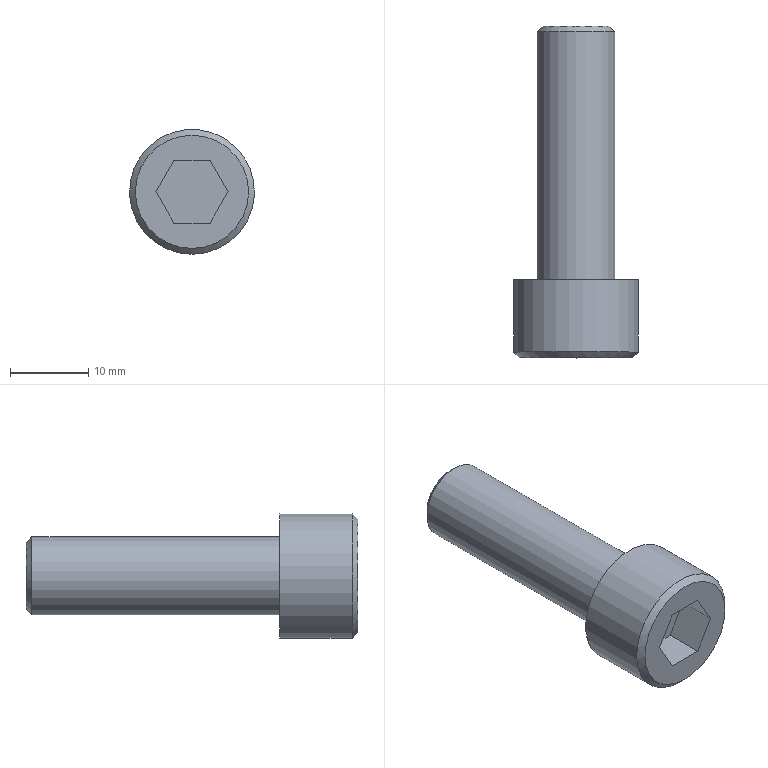Part | STEP file | solid 82 | 1 solid | 14 faces | box 16 x 42.5 x 16 mm | volume 4264 mm3 | plane 10 | cylinder 2 | cone 2 | commonest cylinder face diameters 10 x1 16 x1